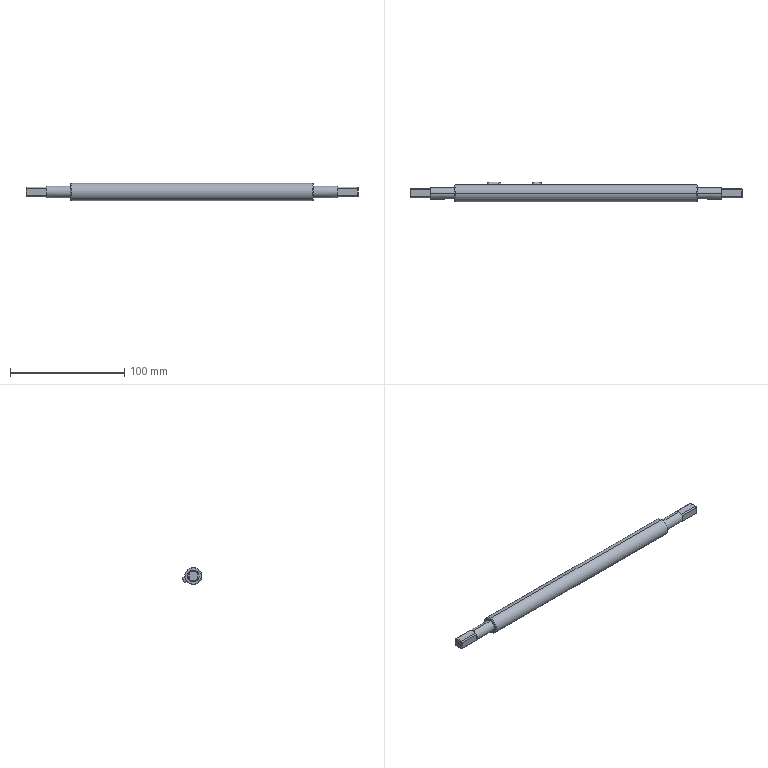Part | SolidWorks | features ICE 3, Chamfer 1, Cut 1, Extrusion 1, Fillet 1, MirrorPattern 1 | 3 solids | 72 faces | box 290 x 17.22 x 15 mm | volume 43172 mm3 | plane 42 | cylinder 18 | cone 12 | commonest cylinder face diameters 5 x12 10 x4 15 x2